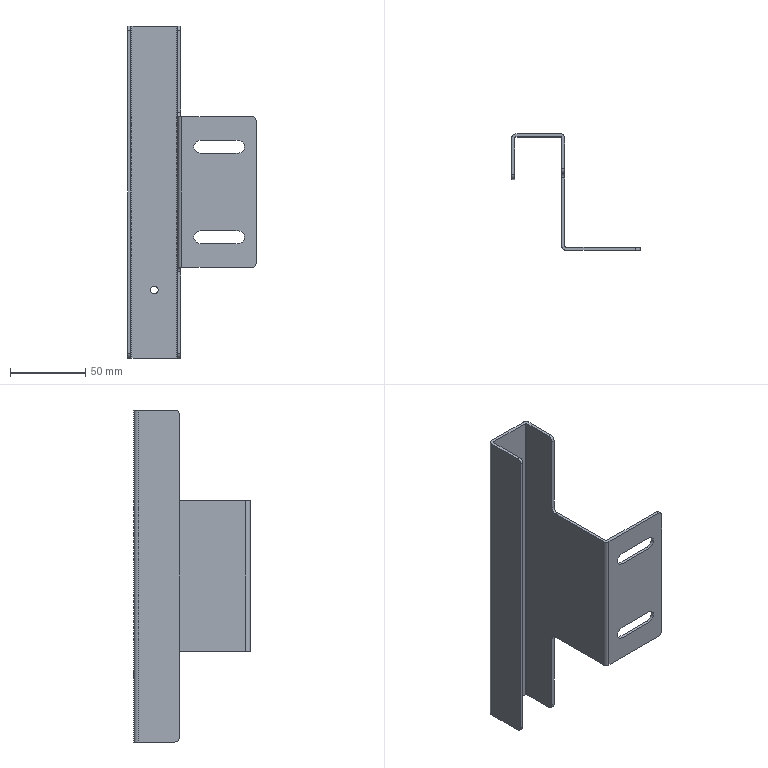Part | SolidWorks | features BaseBody 1 | 1 solid | 40 faces | box 85 x 77 x 220 mm | volume 56604 mm3 | cylinder 20 | plane 20 | commonest cylinder face diameters 6 x8 8.5 x4 1.473 x3 5.473 x3 5 x2
STEP:
#1=CARTESIAN_POINT('',(17.5,-2.,-67.5));
#2=VERTEX_POINT('',#1);
#3=CARTESIAN_POINT('',(17.5,-2.,-62.5));
#4=VERTEX_POINT('',#3);
#5=CARTESIAN_POINT('',(17.5,-2.,-65.));
#6=DIRECTION('',(0.,1.,0.));
#7=DIRECTION('',(0.,0.,1.));
#8=AXIS2_PLACEMENT_3D('',#5,#6,#7);
#9=CIRCLE('',#8,2.5);
#10=EDGE_CURVE('',#2,#4,#9,.T.);
#11=ORIENTED_EDGE('',*,*,#10,.F.);
#12=CARTESIAN_POINT('',(17.5,0.,-67.5));
#13=VERTEX_POINT('',#12);
#14=CARTESIAN_POINT('',(17.5,-10.,-67.5));
#15=DIRECTION('',(0.,1.,0.));
#16=VECTOR('',#15,1000.);
#17=LINE('',#14,#16);
#18=EDGE_CURVE('',#2,#13,#17,.T.);
#19=ORIENTED_EDGE('',*,*,#18,.T.);
#20=CARTESIAN_POINT('',(17.5,0.,-62.5));
#21=VERTEX_POINT('',#20);
#22=CARTESIAN_POINT('',(17.5,0.,-65.));
#23=DIRECTION('',(0.,-1.,0.));
#24=DIRECTION('',(0.,0.,1.));
#25=AXIS2_PLACEMENT_3D('',#22,#23,#24);
#26=CIRCLE('',#25,2.5);
#27=EDGE_CURVE('',#21,#13,#26,.T.);
#28=ORIENTED_EDGE('',*,*,#27,.F.);
#29=CARTESIAN_POINT('',(17.5,-10.,-62.5));
#30=DIRECTION('',(0.,1.,0.));
#31=VECTOR('',#30,1000.);
#32=LINE('',#29,#31);
#33=EDGE_CURVE('',#4,#21,#32,.T.);
#34=ORIENTED_EDGE('',*,*,#33,.F.);
#35=EDGE_LOOP('',(#11,#19,#28,#34));
#36=FACE_OUTER_BOUND('',#35,.T.);
#37=CARTESIAN_POINT('',(17.5,-10.,-65.));
#38=DIRECTION('',(0.,1.,0.));
#39=DIRECTION('',(0.,0.,1.));
#40=AXIS2_PLACEMENT_3D('',#37,#38,#39);
#41=CYLINDRICAL_SURFACE('',#40,2.5);
#42=ADVANCED_FACE('',(#36),#41,.F.);
#43=CARTESIAN_POINT('',(35.,-74.263,-50.));
#44=VERTEX_POINT('',#43);
#45=CARTESIAN_POINT('',(35.,-29.255,-50.));
#46=VERTEX_POINT('',#45);
#47=CARTESIAN_POINT('',(35.,0.,-50.));
#48=DIRECTION('',(0.,1.,0.));
#49=VECTOR('',#48,1000.);
#50=LINE('',#47,#49);
#51=EDGE_CURVE('',#44,#46,#50,.T.);
#52=ORIENTED_EDGE('',*,*,#51,.T.);
#53=CARTESIAN_POINT('',(35.,-26.255,-53.));
#54=VERTEX_POINT('',#53);
#55=CARTESIAN_POINT('',(35.,-29.255,-53.));
#56=DIRECTION('',(-1.,0.,0.));
#57=DIRECTION('',(0.,0.,1.));
#58=AXIS2_PLACEMENT_3D('',#55,#56,#57);
#59=CIRCLE('',#58,3.);
#60=EDGE_CURVE('',#46,#54,#59,.T.);
#61=ORIENTED_EDGE('',*,*,#60,.T.);
#62=CARTESIAN_POINT('',(35.,-26.255,-107.));
#63=VERTEX_POINT('',#62);
#64=CARTESIAN_POINT('',(35.,-26.255,110.));
#65=DIRECTION('',(0.,0.,-1.));
#66=VECTOR('',#65,1000.);
#67=LINE('',#64,#66);
#68=EDGE_CURVE('',#54,#63,#67,.T.);
#69=ORIENTED_EDGE('',*,*,#68,.T.);
#70=CARTESIAN_POINT('',(35.,-23.255,-110.));
#71=VERTEX_POINT('',#70);
#72=CARTESIAN_POINT('',(35.,-23.255,-107.));
#73=DIRECTION('',(1.,0.,0.));
#74=DIRECTION('',(0.,0.,1.));
#75=AXIS2_PLACEMENT_3D('',#72,#73,#74);
#76=CIRCLE('',#75,3.);
#77=EDGE_CURVE('',#63,#71,#76,.T.);
#78=ORIENTED_EDGE('',*,*,#77,.T.);
#79=CARTESIAN_POINT('',(35.,-2.737,-110.));
#80=VERTEX_POINT('',#79);
#81=CARTESIAN_POINT('',(35.,0.,-110.));
#82=DIRECTION('',(0.,1.,0.));
#83=VECTOR('',#82,1000.);
#84=LINE('',#81,#83);
#85=EDGE_CURVE('',#71,#80,#84,.T.);
#86=ORIENTED_EDGE('',*,*,#85,.T.);
#87=CARTESIAN_POINT('',(35.,-2.737,110.));
#88=VERTEX_POINT('',#87);
#89=CARTESIAN_POINT('',(35.,-2.737,110.));
#90=DIRECTION('',(0.,0.,1.));
#91=VECTOR('',#90,1000.);
#92=LINE('',#89,#91);
#93=EDGE_CURVE('',#80,#88,#92,.T.);
#94=ORIENTED_EDGE('',*,*,#93,.T.);
#95=CARTESIAN_POINT('',(35.,-23.255,110.));
#96=VERTEX_POINT('',#95);
#97=CARTESIAN_POINT('',(35.,0.,110.));
#98=DIRECTION('',(0.,-1.,0.));
#99=VECTOR('',#98,1000.);
#100=LINE('',#97,#99);
#101=EDGE_CURVE('',#88,#96,#100,.T.);
#102=ORIENTED_EDGE('',*,*,#101,.T.);
#103=CARTESIAN_POINT('',(35.,-26.255,107.));
#104=VERTEX_POINT('',#103);
#105=CARTESIAN_POINT('',(35.,-23.255,107.));
#106=DIRECTION('',(1.,0.,0.));
#107=DIRECTION('',(0.,0.,1.));
#108=AXIS2_PLACEMENT_3D('',#105,#106,#107);
#109=CIRCLE('',#108,3.);
#110=EDGE_CURVE('',#96,#104,#109,.T.);
#111=ORIENTED_EDGE('',*,*,#110,.T.);
#112=CARTESIAN_POINT('',(35.,-26.255,53.));
#113=VERTEX_POINT('',#112);
#114=CARTESIAN_POINT('',(35.,-26.255,110.));
#115=DIRECTION('',(0.,0.,-1.));
#116=VECTOR('',#115,1000.);
#117=LINE('',#114,#116);
#118=EDGE_CURVE('',#104,#113,#117,.T.);
#119=ORIENTED_EDGE('',*,*,#118,.T.);
#120=CARTESIAN_POINT('',(35.,-29.255,50.));
#121=VERTEX_POINT('',#120);
#122=CARTESIAN_POINT('',(35.,-29.255,53.));
#123=DIRECTION('',(-1.,0.,0.));
#124=DIRECTION('',(0.,0.,1.));
#125=AXIS2_PLACEMENT_3D('',#122,#123,#124);
#126=CIRCLE('',#125,3.);
#127=EDGE_CURVE('',#113,#121,#126,.T.);
#128=ORIENTED_EDGE('',*,*,#127,.T.);
#129=CARTESIAN_POINT('',(35.,-74.263,50.));
#130=VERTEX_POINT('',#129);
#131=CARTESIAN_POINT('',(35.,0.,50.));
#132=DIRECTION('',(0.,-1.,0.));
#133=VECTOR('',#132,1000.);
#134=LINE('',#131,#133);
#135=EDGE_CURVE('',#121,#130,#134,.T.);
#136=ORIENTED_EDGE('',*,*,#135,.T.);
#137=CARTESIAN_POINT('',(35.,-74.263,110.));
#138=DIRECTION('',(0.,0.,-1.));
#139=VECTOR('',#138,1000.);
#140=LINE('',#137,#139);
#141=EDGE_CURVE('',#130,#44,#140,.T.);
#142=ORIENTED_EDGE('',*,*,#141,.T.);
#143=EDGE_LOOP('',(#52,#61,#69,#78,#86,#94,#102,#111,#119,#128,#136,#142));
#144=FACE_OUTER_BOUND('',#143,.T.);
#145=CARTESIAN_POINT('',(35.,0.,110.));
#146=DIRECTION('',(1.,0.,0.));
#147=DIRECTION('',(0.,0.,-1.));
#148=AXIS2_PLACEMENT_3D('',#145,#146,#147);
#149=PLANE('',#148);
#150=ADVANCED_FACE('',(#144),#149,.T.);
#151=CARTESIAN_POINT('',(33.,-26.255,-53.));
#152=VERTEX_POINT('',#151);
#153=CARTESIAN_POINT('',(25.,-26.255,-53.));
#154=DIRECTION('',(-1.,0.,0.));
#155=VECTOR('',#154,1000.);
#156=LINE('',#153,#155);
#157=EDGE_CURVE('',#54,#152,#156,.T.);
#158=ORIENTED_EDGE('',*,*,#157,.F.);
#159=ORIENTED_EDGE('',*,*,#60,.F.);
#160=CARTESIAN_POINT('',(33.,-29.255,-50.));
#161=VERTEX_POINT('',#160);
#162=CARTESIAN_POINT('',(25.,-29.255,-50.));
#163=DIRECTION('',(1.,0.,0.));
#164=VECTOR('',#163,1000.);
#165=LINE('',#162,#164);
#166=EDGE_CURVE('',#161,#46,#165,.T.);
#167=ORIENTED_EDGE('',*,*,#166,.F.);
#168=CARTESIAN_POINT('',(33.,-29.255,-53.));
#169=DIRECTION('',(1.,0.,0.));
#170=DIRECTION('',(0.,0.,1.));
#171=AXIS2_PLACEMENT_3D('',#168,#169,#170);
#172=CIRCLE('',#171,3.);
#173=EDGE_CURVE('',#152,#161,#172,.T.);
#174=ORIENTED_EDGE('',*,*,#173,.F.);
#175=EDGE_LOOP('',(#158,#159,#167,#174));
#176=FACE_OUTER_BOUND('',#175,.T.);
#177=CARTESIAN_POINT('',(25.,-29.255,-53.));
#178=DIRECTION('',(-1.,0.,0.));
#179=DIRECTION('',(0.,0.,1.));
#180=AXIS2_PLACEMENT_3D('',#177,#178,#179);
#181=CYLINDRICAL_SURFACE('',#180,3.);
#182=ADVANCED_FACE('',(#176),#181,.F.);
#183=ORIENTED_EDGE('',*,*,#166,.T.);
#184=ORIENTED_EDGE('',*,*,#51,.F.);
#185=CARTESIAN_POINT('',(35.737,-75.,-50.));
#186=VERTEX_POINT('',#185);
#187=CARTESIAN_POINT('',(35.737,-74.263,-50.));
#188=DIRECTION('',(0.,0.,1.));
#189=DIRECTION('',(-1.,0.,0.));
#190=AXIS2_PLACEMENT_3D('',#187,#188,#189);
#191=CIRCLE('',#190,0.7366);
#192=EDGE_CURVE('',#44,#186,#191,.T.);
#193=ORIENTED_EDGE('',*,*,#192,.T.);
#194=CARTESIAN_POINT('',(82.,-75.,-50.));
#195=VERTEX_POINT('',#194);
#196=CARTESIAN_POINT('',(35.,-75.,-50.));
#197=DIRECTION('',(-1.,0.,0.));
#198=VECTOR('',#197,1000.);
#199=LINE('',#196,#198);
#200=EDGE_CURVE('',#195,#186,#199,.T.);
#201=ORIENTED_EDGE('',*,*,#200,.F.);
#202=CARTESIAN_POINT('',(82.,-77.,-50.));
#203=VERTEX_POINT('',#202);
#204=CARTESIAN_POINT('',(82.,-85.,-50.));
#205=DIRECTION('',(0.,1.,0.));
#206=VECTOR('',#205,1000.);
#207=LINE('',#204,#206);
#208=EDGE_CURVE('',#203,#195,#207,.T.);
#209=ORIENTED_EDGE('',*,*,#208,.F.);
#210=CARTESIAN_POINT('',(35.737,-77.,-50.));
#211=VERTEX_POINT('',#210);
#212=CARTESIAN_POINT('',(85.,-77.,-50.));
#213=DIRECTION('',(1.,0.,0.));
#214=VECTOR('',#213,1000.);
#215=LINE('',#212,#214);
#216=EDGE_CURVE('',#211,#203,#215,.T.);
#217=ORIENTED_EDGE('',*,*,#216,.F.);
#218=CARTESIAN_POINT('',(33.,-74.263,-50.));
#219=VERTEX_POINT('',#218);
#220=CARTESIAN_POINT('',(35.737,-74.263,-50.));
#221=DIRECTION('',(0.,0.,1.));
#222=DIRECTION('',(-1.,0.,0.));
#223=AXIS2_PLACEMENT_3D('',#220,#221,#222);
#224=CIRCLE('',#223,2.737);
#225=EDGE_CURVE('',#219,#211,#224,.T.);
#226=ORIENTED_EDGE('',*,*,#225,.F.);
#227=CARTESIAN_POINT('',(33.,-126.255,-50.));
#228=DIRECTION('',(0.,-1.,0.));
#229=VECTOR('',#228,1000.);
#230=LINE('',#227,#229);
#231=EDGE_CURVE('',#161,#219,#230,.T.);
#232=ORIENTED_EDGE('',*,*,#231,.F.);
#233=EDGE_LOOP('',(#183,#184,#193,#201,#209,#217,#226,#232));
#234=FACE_OUTER_BOUND('',#233,.T.);
#235=CARTESIAN_POINT('',(25.,-126.255,-50.));
#236=DIRECTION('',(0.,0.,1.));
#237=DIRECTION('',(1.,0.,0.));
#238=AXIS2_PLACEMENT_3D('',#235,#236,#237);
#239=PLANE('',#238);
#240=ADVANCED_FACE('',(#234),#239,.F.);
#241=ORIENTED_EDGE('',*,*,#141,.F.);
#242=CARTESIAN_POINT('',(35.737,-75.,50.));
#243=VERTEX_POINT('',#242);
#244=CARTESIAN_POINT('',(35.737,-74.263,50.));
#245=DIRECTION('',(0.,0.,1.));
#246=DIRECTION('',(-1.,0.,0.));
#247=AXIS2_PLACEMENT_3D('',#244,#245,#246);
#248=CIRCLE('',#247,0.7366);
#249=EDGE_CURVE('',#130,#243,#248,.T.);
#250=ORIENTED_EDGE('',*,*,#249,.T.);
#251=CARTESIAN_POINT('',(35.737,-75.,100.057));
#252=DIRECTION('',(0.,0.,1.));
#253=VECTOR('',#252,1000.);
#254=LINE('',#251,#253);
#255=EDGE_CURVE('',#186,#243,#254,.T.);
#256=ORIENTED_EDGE('',*,*,#255,.F.);
#257=ORIENTED_EDGE('',*,*,#192,.F.);
#258=EDGE_LOOP('',(#241,#250,#256,#257));
#259=FACE_OUTER_BOUND('',#258,.T.);
#260=CARTESIAN_POINT('',(35.737,-74.263,100.057));
#261=DIRECTION('',(0.,0.,-1.));
#262=DIRECTION('',(-1.,0.,0.));
#263=AXIS2_PLACEMENT_3D('',#260,#261,#262);
#264=CYLINDRICAL_SURFACE('',#263,0.7366);
#265=ADVANCED_FACE('',(#259),#264,.F.);
#266=CARTESIAN_POINT('',(33.,-29.255,50.));
#267=VERTEX_POINT('',#266);
#268=CARTESIAN_POINT('',(25.,-29.255,50.));
#269=DIRECTION('',(1.,0.,0.));
#270=VECTOR('',#269,1000.);
#271=LINE('',#268,#270);
#272=EDGE_CURVE('',#267,#121,#271,.T.);
#273=ORIENTED_EDGE('',*,*,#272,.F.);
#274=CARTESIAN_POINT('',(33.,-74.263,50.));
#275=VERTEX_POINT('',#274);
#276=CARTESIAN_POINT('',(33.,-126.255,50.));
#277=DIRECTION('',(0.,1.,0.));
#278=VECTOR('',#277,1000.);
#279=LINE('',#276,#278);
#280=EDGE_CURVE('',#275,#267,#279,.T.);
#281=ORIENTED_EDGE('',*,*,#280,.F.);
#282=CARTESIAN_POINT('',(35.737,-77.,50.));
#283=VERTEX_POINT('',#282);
#284=CARTESIAN_POINT('',(35.737,-74.263,50.));
#285=DIRECTION('',(0.,0.,-1.));
#286=DIRECTION('',(-1.,0.,0.));
#287=AXIS2_PLACEMENT_3D('',#284,#285,#286);
#288=CIRCLE('',#287,2.737);
#289=EDGE_CURVE('',#283,#275,#288,.T.);
#290=ORIENTED_EDGE('',*,*,#289,.F.);
#291=CARTESIAN_POINT('',(82.,-77.,50.));
#292=VERTEX_POINT('',#291);
#293=CARTESIAN_POINT('',(85.,-77.,50.));
#294=DIRECTION('',(-1.,0.,0.));
#295=VECTOR('',#294,1000.);
#296=LINE('',#293,#295);
#297=EDGE_CURVE('',#292,#283,#296,.T.);
#298=ORIENTED_EDGE('',*,*,#297,.F.);
#299=CARTESIAN_POINT('',(82.,-75.,50.));
#300=VERTEX_POINT('',#299);
#301=CARTESIAN_POINT('',(82.,-85.,50.));
#302=DIRECTION('',(0.,-1.,0.));
#303=VECTOR('',#302,1000.);
#304=LINE('',#301,#303);
#305=EDGE_CURVE('',#300,#292,#304,.T.);
#306=ORIENTED_EDGE('',*,*,#305,.F.);
#307=CARTESIAN_POINT('',(35.,-75.,50.));
#308=DIRECTION('',(1.,0.,0.));
#309=VECTOR('',#308,1000.);
#310=LINE('',#307,#309);
#311=EDGE_CURVE('',#243,#300,#310,.T.);
#312=ORIENTED_EDGE('',*,*,#311,.F.);
#313=ORIENTED_EDGE('',*,*,#249,.F.);
#314=ORIENTED_EDGE('',*,*,#135,.F.);
#315=EDGE_LOOP('',(#273,#281,#290,#298,#306,#312,#313,#314));
#316=FACE_OUTER_BOUND('',#315,.T.);
#317=CARTESIAN_POINT('',(25.,-126.255,50.));
#318=DIRECTION('',(0.,0.,-1.));
#319=DIRECTION('',(0.,1.,0.));
#320=AXIS2_PLACEMENT_3D('',#317,#318,#319);
#321=PLANE('',#320);
#322=ADVANCED_FACE('',(#316),#321,.F.);
#323=ORIENTED_EDGE('',*,*,#272,.T.);
#324=ORIENTED_EDGE('',*,*,#127,.F.);
#325=CARTESIAN_POINT('',(33.,-26.255,53.));
#326=VERTEX_POINT('',#325);
#327=CARTESIAN_POINT('',(25.,-26.255,53.));
#328=DIRECTION('',(1.,0.,0.));
#329=VECTOR('',#328,1000.);
#330=LINE('',#327,#329);
#331=EDGE_CURVE('',#326,#113,#330,.T.);
#332=ORIENTED_EDGE('',*,*,#331,.F.);
#333=CARTESIAN_POINT('',(33.,-29.255,53.));
#334=DIRECTION('',(1.,0.,0.));
#335=DIRECTION('',(0.,0.,1.));
#336=AXIS2_PLACEMENT_3D('',#333,#334,#335);
#337=CIRCLE('',#336,3.);
#338=EDGE_CURVE('',#267,#326,#337,.T.);
#339=ORIENTED_EDGE('',*,*,#338,.F.);
#340=EDGE_LOOP('',(#323,#324,#332,#339));
#341=FACE_OUTER_BOUND('',#340,.T.);
#342=CARTESIAN_POINT('',(25.,-29.255,53.));
#343=DIRECTION('',(-1.,0.,0.));
#344=DIRECTION('',(0.,0.,1.));
#345=AXIS2_PLACEMENT_3D('',#342,#343,#344);
#346=CYLINDRICAL_SURFACE('',#345,3.);
#347=ADVANCED_FACE('',(#341),#346,.F.);
#348=ORIENTED_EDGE('',*,*,#331,.T.);
#349=ORIENTED_EDGE('',*,*,#118,.F.);
#350=CARTESIAN_POINT('',(33.,-26.255,107.));
#351=VERTEX_POINT('',#350);
#352=CARTESIAN_POINT('',(25.,-26.255,107.));
#353=DIRECTION('',(1.,0.,0.));
#354=VECTOR('',#353,1000.);
#355=LINE('',#352,#354);
#356=EDGE_CURVE('',#351,#104,#355,.T.);
#357=ORIENTED_EDGE('',*,*,#356,.F.);
#358=CARTESIAN_POINT('',(33.,-26.255,110.));
#359=DIRECTION('',(0.,0.,1.));
#360=VECTOR('',#359,1000.);
#361=LINE('',#358,#360);
#362=EDGE_CURVE('',#326,#351,#361,.T.);
#363=ORIENTED_EDGE('',*,*,#362,.F.);
#364=EDGE_LOOP('',(#348,#349,#357,#363));
#365=FACE_OUTER_BOUND('',#364,.T.);
#366=CARTESIAN_POINT('',(25.,-26.255,110.));
#367=DIRECTION('',(0.,1.,0.));
#368=DIRECTION('',(0.,0.,1.));
#369=AXIS2_PLACEMENT_3D('',#366,#367,#368);
#370=PLANE('',#369);
#371=ADVANCED_FACE('',(#365),#370,.F.);
#372=ORIENTED_EDGE('',*,*,#110,.F.);
#373=CARTESIAN_POINT('',(33.,-23.255,110.));
#374=VERTEX_POINT('',#373);
#375=CARTESIAN_POINT('',(32.263,-23.255,110.));
#376=DIRECTION('',(-1.,0.,0.));
#377=VECTOR('',#376,1000.);
#378=LINE('',#375,#377);
#379=EDGE_CURVE('',#96,#374,#378,.T.);
#380=ORIENTED_EDGE('',*,*,#379,.T.);
#381=CARTESIAN_POINT('',(33.,-23.255,107.));
#382=DIRECTION('',(1.,0.,0.));
#383=DIRECTION('',(0.,0.,1.));
#384=AXIS2_PLACEMENT_3D('',#381,#382,#383);
#385=CIRCLE('',#384,3.);
#386=EDGE_CURVE('',#374,#351,#385,.T.);
#387=ORIENTED_EDGE('',*,*,#386,.T.);
#388=ORIENTED_EDGE('',*,*,#356,.T.);
#389=EDGE_LOOP('',(#372,#380,#387,#388));
#390=FACE_OUTER_BOUND('',#389,.T.);
#391=CARTESIAN_POINT('',(32.263,-23.255,107.));
#392=DIRECTION('',(-1.,0.,0.));
#393=DIRECTION('',(0.,0.,1.));
#394=AXIS2_PLACEMENT_3D('',#391,#392,#393);
#395=CYLINDRICAL_SURFACE('',#394,3.);
#396=ADVANCED_FACE('',(#390),#395,.T.);
#397=ORIENTED_EDGE('',*,*,#101,.F.);
#398=CARTESIAN_POINT('',(32.263,0.,110.));
#399=VERTEX_POINT('',#398);
#400=CARTESIAN_POINT('',(32.263,-2.737,110.));
#401=DIRECTION('',(0.,0.,-1.));
#402=DIRECTION('',(-1.,0.,0.));
#403=AXIS2_PLACEMENT_3D('',#400,#401,#402);
#404=CIRCLE('',#403,2.737);
#405=EDGE_CURVE('',#399,#88,#404,.T.);
#406=ORIENTED_EDGE('',*,*,#405,.F.);
#407=CARTESIAN_POINT('',(2.737,0.,110.));
#408=VERTEX_POINT('',#407);
#409=CARTESIAN_POINT('',(0.,0.,110.));
#410=DIRECTION('',(1.,0.,0.));
#411=VECTOR('',#410,1000.);
#412=LINE('',#409,#411);
#413=EDGE_CURVE('',#408,#399,#412,.T.);
#414=ORIENTED_EDGE('',*,*,#413,.F.);
#415=CARTESIAN_POINT('',(0.,-2.737,110.));
#416=VERTEX_POINT('',#415);
#417=CARTESIAN_POINT('',(2.737,-2.737,110.));
#418=DIRECTION('',(0.,0.,-1.));
#419=DIRECTION('',(-1.,0.,0.));
#420=AXIS2_PLACEMENT_3D('',#417,#418,#419);
#421=CIRCLE('',#420,2.737);
#422=EDGE_CURVE('',#416,#408,#421,.T.);
#423=ORIENTED_EDGE('',*,*,#422,.F.);
#424=CARTESIAN_POINT('',(0.,-27.,110.));
#425=VERTEX_POINT('',#424);
#426=CARTESIAN_POINT('',(0.,-30.,110.));
#427=DIRECTION('',(0.,1.,0.));
#428=VECTOR('',#427,1000.);
#429=LINE('',#426,#428);
#430=EDGE_CURVE('',#425,#416,#429,.T.);
#431=ORIENTED_EDGE('',*,*,#430,.F.);
#432=CARTESIAN_POINT('',(2.,-27.,110.));
#433=VERTEX_POINT('',#432);
#434=CARTESIAN_POINT('',(35.737,-27.,110.));
#435=DIRECTION('',(-1.,0.,0.));
#436=VECTOR('',#435,1000.);
#437=LINE('',#434,#436);
#438=EDGE_CURVE('',#433,#425,#437,.T.);
#439=ORIENTED_EDGE('',*,*,#438,.F.);
#440=CARTESIAN_POINT('',(2.,-2.737,110.));
#441=VERTEX_POINT('',#440);
#442=CARTESIAN_POINT('',(2.,-74.263,110.));
#443=DIRECTION('',(0.,-1.,0.));
#444=VECTOR('',#443,1000.);
#445=LINE('',#442,#444);
#446=EDGE_CURVE('',#441,#433,#445,.T.);
#447=ORIENTED_EDGE('',*,*,#446,.F.);
#448=CARTESIAN_POINT('',(2.737,-2.,110.));
#449=VERTEX_POINT('',#448);
#450=CARTESIAN_POINT('',(2.737,-2.737,110.));
#451=DIRECTION('',(0.,0.,-1.));
#452=DIRECTION('',(-1.,0.,0.));
#453=AXIS2_PLACEMENT_3D('',#450,#451,#452);
#454=CIRCLE('',#453,0.7366);
#455=EDGE_CURVE('',#441,#449,#454,.T.);
#456=ORIENTED_EDGE('',*,*,#455,.T.);
#457=CARTESIAN_POINT('',(32.263,-2.,110.));
#458=VERTEX_POINT('',#457);
#459=CARTESIAN_POINT('',(2.,-2.,110.));
#460=DIRECTION('',(1.,0.,0.));
#461=VECTOR('',#460,1000.);
#462=LINE('',#459,#461);
#463=EDGE_CURVE('',#449,#458,#462,.T.);
#464=ORIENTED_EDGE('',*,*,#463,.T.);
#465=CARTESIAN_POINT('',(33.,-2.737,110.));
#466=VERTEX_POINT('',#465);
#467=CARTESIAN_POINT('',(32.263,-2.737,110.));
#468=DIRECTION('',(0.,0.,-1.));
#469=DIRECTION('',(-1.,0.,0.));
#470=AXIS2_PLACEMENT_3D('',#467,#468,#469);
#471=CIRCLE('',#470,0.7366);
#472=EDGE_CURVE('',#458,#466,#471,.T.);
#473=ORIENTED_EDGE('',*,*,#472,.T.);
#474=CARTESIAN_POINT('',(33.,-2.,110.));
#475=DIRECTION('',(0.,-1.,0.));
#476=VECTOR('',#475,1000.);
#477=LINE('',#474,#476);
#478=EDGE_CURVE('',#466,#374,#477,.T.);
#479=ORIENTED_EDGE('',*,*,#478,.T.);
#480=ORIENTED_EDGE('',*,*,#379,.F.);
#481=EDGE_LOOP('',(#397,#406,#414,#423,#431,#439,#447,#456,#464,#473,#479,#480));
#482=FACE_OUTER_BOUND('',#481,.T.);
#483=CARTESIAN_POINT('',(32.263,-2.,110.));
#484=DIRECTION('',(0.,0.,1.));
#485=DIRECTION('',(1.,0.,0.));
#486=AXIS2_PLACEMENT_3D('',#483,#484,#485);
#487=PLANE('',#486);
#488=ADVANCED_FACE('',(#482),#487,.T.);
#489=ORIENTED_EDGE('',*,*,#405,.T.);
#490=ORIENTED_EDGE('',*,*,#93,.F.);
#491=CARTESIAN_POINT('',(32.263,0.,-110.));
#492=VERTEX_POINT('',#491);
#493=CARTESIAN_POINT('',(32.263,-2.737,-110.));
#494=DIRECTION('',(0.,0.,1.));
#495=DIRECTION('',(-1.,0.,0.));
#496=AXIS2_PLACEMENT_3D('',#493,#494,#495);
#497=CIRCLE('',#496,2.737);
#498=EDGE_CURVE('',#80,#492,#497,.T.);
#499=ORIENTED_EDGE('',*,*,#498,.T.);
#500=CARTESIAN_POINT('',(32.263,0.,110.));
#501=DIRECTION('',(0.,0.,1.));
#502=VECTOR('',#501,1000.);
#503=LINE('',#500,#502);
#504=EDGE_CURVE('',#492,#399,#503,.T.);
#505=ORIENTED_EDGE('',*,*,#504,.T.);
#506=EDGE_LOOP('',(#489,#490,#499,#505));
#507=FACE_OUTER_BOUND('',#506,.T.);
#508=CARTESIAN_POINT('',(32.263,-2.737,110.));
#509=DIRECTION('',(0.,0.,-1.));
#510=DIRECTION('',(-1.,0.,0.));
#511=AXIS2_PLACEMENT_3D('',#508,#509,#510);
#512=CYLINDRICAL_SURFACE('',#511,2.737);
#513=ADVANCED_FACE('',(#507),#512,.T.);
#514=CARTESIAN_POINT('',(33.,-23.255,-110.));
#515=VERTEX_POINT('',#514);
#516=CARTESIAN_POINT('',(33.,-2.737,-110.));
#517=VERTEX_POINT('',#516);
#518=CARTESIAN_POINT('',(33.,-77.,-110.));
#519=DIRECTION('',(0.,1.,0.));
#520=VECTOR('',#519,1000.);
#521=LINE('',#518,#520);
#522=EDGE_CURVE('',#515,#517,#521,.T.);
#523=ORIENTED_EDGE('',*,*,#522,.T.);
#524=CARTESIAN_POINT('',(32.263,-2.,-110.));
#525=VERTEX_POINT('',#524);
#526=CARTESIAN_POINT('',(32.263,-2.737,-110.));
#527=DIRECTION('',(0.,0.,1.));
#528=DIRECTION('',(-1.,0.,0.));
#529=AXIS2_PLACEMENT_3D('',#526,#527,#528);
#530=CIRCLE('',#529,0.7366);
#531=EDGE_CURVE('',#517,#525,#530,.T.);
#532=ORIENTED_EDGE('',*,*,#531,.T.);
#533=CARTESIAN_POINT('',(2.737,-2.,-110.));
#534=VERTEX_POINT('',#533);
#535=CARTESIAN_POINT('',(33.,-2.,-110.));
#536=DIRECTION('',(-1.,0.,0.));
#537=VECTOR('',#536,1000.);
#538=LINE('',#535,#537);
#539=EDGE_CURVE('',#525,#534,#538,.T.);
#540=ORIENTED_EDGE('',*,*,#539,.T.);
#541=CARTESIAN_POINT('',(2.,-2.737,-110.));
#542=VERTEX_POINT('',#541);
#543=CARTESIAN_POINT('',(2.737,-2.737,-110.));
#544=DIRECTION('',(0.,0.,1.));
#545=DIRECTION('',(-1.,0.,0.));
#546=AXIS2_PLACEMENT_3D('',#543,#544,#545);
#547=CIRCLE('',#546,0.7366);
#548=EDGE_CURVE('',#534,#542,#547,.T.);
#549=ORIENTED_EDGE('',*,*,#548,.T.);
#550=CARTESIAN_POINT('',(2.,-27.,-110.));
#551=VERTEX_POINT('',#550);
#552=CARTESIAN_POINT('',(2.,-2.,-110.));
#553=DIRECTION('',(0.,-1.,0.));
#554=VECTOR('',#553,1000.);
#555=LINE('',#552,#554);
#556=EDGE_CURVE('',#542,#551,#555,.T.);
#557=ORIENTED_EDGE('',*,*,#556,.T.);
#558=CARTESIAN_POINT('',(0.,-27.,-110.));
#559=VERTEX_POINT('',#558);
#560=CARTESIAN_POINT('',(2.737,-27.,-110.));
#561=DIRECTION('',(1.,0.,0.));
#562=VECTOR('',#561,1000.);
#563=LINE('',#560,#562);
#564=EDGE_CURVE('',#559,#551,#563,.T.);
#565=ORIENTED_EDGE('',*,*,#564,.F.);
#566=CARTESIAN_POINT('',(0.,-2.737,-110.));
#567=VERTEX_POINT('',#566);
#568=CARTESIAN_POINT('',(0.,-30.,-110.));
#569=DIRECTION('',(0.,-1.,0.));
#570=VECTOR('',#569,1000.);
#571=LINE('',#568,#570);
#572=EDGE_CURVE('',#567,#559,#571,.T.);
#573=ORIENTED_EDGE('',*,*,#572,.F.);
#574=CARTESIAN_POINT('',(2.737,0.,-110.));
#575=VERTEX_POINT('',#574);
#576=CARTESIAN_POINT('',(2.737,-2.737,-110.));
#577=DIRECTION('',(0.,0.,1.));
#578=DIRECTION('',(-1.,0.,0.));
#579=AXIS2_PLACEMENT_3D('',#576,#577,#578);
#580=CIRCLE('',#579,2.737);
#581=EDGE_CURVE('',#575,#567,#580,.T.);
#582=ORIENTED_EDGE('',*,*,#581,.F.);
#583=CARTESIAN_POINT('',(0.,0.,-110.));
#584=DIRECTION('',(-1.,0.,0.));
#585=VECTOR('',#584,1000.);
#586=LINE('',#583,#585);
#587=EDGE_CURVE('',#492,#575,#586,.T.);
#588=ORIENTED_EDGE('',*,*,#587,.F.);
#589=ORIENTED_EDGE('',*,*,#498,.F.);
#590=ORIENTED_EDGE('',*,*,#85,.F.);
#591=CARTESIAN_POINT('',(35.737,-23.255,-110.));
#592=DIRECTION('',(-1.,0.,0.));
#593=VECTOR('',#592,1000.);
#594=LINE('',#591,#593);
#595=EDGE_CURVE('',#71,#515,#594,.T.);
#596=ORIENTED_EDGE('',*,*,#595,.T.);
#597=EDGE_LOOP('',(#523,#532,#540,#549,#557,#565,#573,#582,#588,#589,#590,#596));
#598=FACE_OUTER_BOUND('',#597,.T.);
#599=CARTESIAN_POINT('',(35.737,-77.,-110.));
#600=DIRECTION('',(0.,0.,-1.));
#601=DIRECTION('',(-1.,0.,0.));
#602=AXIS2_PLACEMENT_3D('',#599,#600,#601);
#603=PLANE('',#602);
#604=ADVANCED_FACE('',(#598),#603,.T.);
#605=ORIENTED_EDGE('',*,*,#77,.F.);
#606=CARTESIAN_POINT('',(33.,-26.255,-107.));
#607=VERTEX_POINT('',#606);
#608=CARTESIAN_POINT('',(25.,-26.255,-107.));
#609=DIRECTION('',(-1.,0.,0.));
#610=VECTOR('',#609,1000.);
#611=LINE('',#608,#610);
#612=EDGE_CURVE('',#63,#607,#611,.T.);
#613=ORIENTED_EDGE('',*,*,#612,.T.);
#614=CARTESIAN_POINT('',(33.,-23.255,-107.));
#615=DIRECTION('',(1.,0.,0.));
#616=DIRECTION('',(0.,0.,1.));
#617=AXIS2_PLACEMENT_3D('',#614,#615,#616);
#618=CIRCLE('',#617,3.);
#619=EDGE_CURVE('',#607,#515,#618,.T.);
#620=ORIENTED_EDGE('',*,*,#619,.T.);
#621=ORIENTED_EDGE('',*,*,#595,.F.);
#622=EDGE_LOOP('',(#605,#613,#620,#621));
#623=FACE_OUTER_BOUND('',#622,.T.);
#624=CARTESIAN_POINT('',(25.,-23.255,-107.));
#625=DIRECTION('',(-1.,0.,0.));
#626=DIRECTION('',(0.,0.,1.));
#627=AXIS2_PLACEMENT_3D('',#624,#625,#626);
#628=CYLINDRICAL_SURFACE('',#627,3.);
#629=ADVANCED_FACE('',(#623),#628,.T.);
#630=ORIENTED_EDGE('',*,*,#612,.F.);
#631=ORIENTED_EDGE('',*,*,#68,.F.);
#632=ORIENTED_EDGE('',*,*,#157,.T.);
#633=CARTESIAN_POINT('',(33.,-26.255,-110.));
#634=DIRECTION('',(0.,0.,1.));
#635=VECTOR('',#634,1000.);
#636=LINE('',#633,#635);
#637=EDGE_CURVE('',#607,#152,#636,.T.);
#638=ORIENTED_EDGE('',*,*,#637,.F.);
#639=EDGE_LOOP('',(#630,#631,#632,#638));
#640=FACE_OUTER_BOUND('',#639,.T.);
#641=CARTESIAN_POINT('',(25.,-26.255,-110.));
#642=DIRECTION('',(0.,1.,0.));
#643=DIRECTION('',(0.,0.,1.));
#644=AXIS2_PLACEMENT_3D('',#641,#642,#643);
#645=PLANE('',#644);
#646=ADVANCED_FACE('',(#640),#645,.F.);
#647=ORIENTED_EDGE('',*,*,#619,.F.);
#648=ORIENTED_EDGE('',*,*,#637,.T.);
#649=ORIENTED_EDGE('',*,*,#173,.T.);
#650=ORIENTED_EDGE('',*,*,#231,.T.);
#651=CARTESIAN_POINT('',(33.,-74.263,110.));
#652=DIRECTION('',(0.,0.,-1.));
#653=VECTOR('',#652,1000.);
#654=LINE('',#651,#653);
#655=EDGE_CURVE('',#275,#219,#654,.T.);
#656=ORIENTED_EDGE('',*,*,#655,.F.);
#657=ORIENTED_EDGE('',*,*,#280,.T.);
#658=ORIENTED_EDGE('',*,*,#338,.T.);
#659=ORIENTED_EDGE('',*,*,#362,.T.);
#660=ORIENTED_EDGE('',*,*,#386,.F.);
#661=ORIENTED_EDGE('',*,*,#478,.F.);
#662=CARTESIAN_POINT('',(33.,-2.737,110.));
#663=DIRECTION('',(0.,0.,1.));
#664=VECTOR('',#663,1000.);
#665=LINE('',#662,#664);
#666=EDGE_CURVE('',#517,#466,#665,.T.);
#667=ORIENTED_EDGE('',*,*,#666,.F.);
#668=ORIENTED_EDGE('',*,*,#522,.F.);
#669=EDGE_LOOP('',(#647,#648,#649,#650,#656,#657,#658,#659,#660,#661,#667,#668));
#670=FACE_OUTER_BOUND('',#669,.T.);
#671=CARTESIAN_POINT('',(33.,0.,110.));
#672=DIRECTION('',(1.,0.,0.));
#673=DIRECTION('',(0.,0.,-1.));
#674=AXIS2_PLACEMENT_3D('',#671,#672,#673);
#675=PLANE('',#674);
#676=ADVANCED_FACE('',(#670),#675,.F.);
#677=ORIENTED_EDGE('',*,*,#311,.T.);
#678=CARTESIAN_POINT('',(85.,-75.,47.));
#679=VERTEX_POINT('',#678);
#680=CARTESIAN_POINT('',(82.,-75.,47.));
#681=DIRECTION('',(0.,1.,0.));
#682=DIRECTION('',(0.,0.,-1.));
#683=AXIS2_PLACEMENT_3D('',#680,#681,#682);
#684=CIRCLE('',#683,3.);
#685=EDGE_CURVE('',#300,#679,#684,.T.);
#686=ORIENTED_EDGE('',*,*,#685,.T.);
#687=CARTESIAN_POINT('',(85.,-75.,-47.));
#688=VERTEX_POINT('',#687);
#689=CARTESIAN_POINT('',(85.,-75.,110.));
#690=DIRECTION('',(0.,0.,-1.));
#691=VECTOR('',#690,1000.);
#692=LINE('',#689,#691);
#693=EDGE_CURVE('',#679,#688,#692,.T.);
#694=ORIENTED_EDGE('',*,*,#693,.T.);
#695=CARTESIAN_POINT('',(82.,-75.,-47.));
#696=DIRECTION('',(0.,1.,0.));
#697=DIRECTION('',(0.,0.,-1.));
#698=AXIS2_PLACEMENT_3D('',#695,#696,#697);
#699=CIRCLE('',#698,3.);
#700=EDGE_CURVE('',#688,#195,#699,.T.);
#701=ORIENTED_EDGE('',*,*,#700,.T.);
#702=ORIENTED_EDGE('',*,*,#200,.T.);
#703=ORIENTED_EDGE('',*,*,#255,.T.);
#704=EDGE_LOOP('',(#677,#686,#694,#701,#702,#703));
#705=FACE_OUTER_BOUND('',#704,.T.);
#706=CARTESIAN_POINT('',(73.,-75.,25.75));
#707=VERTEX_POINT('',#706);
#708=CARTESIAN_POINT('',(73.,-75.,34.25));
#709=VERTEX_POINT('',#708);
#710=CARTESIAN_POINT('',(73.,-75.,30.));
#711=DIRECTION('',(0.,-1.,0.));
#712=DIRECTION('',(0.,0.,1.));
#713=AXIS2_PLACEMENT_3D('',#710,#711,#712);
#714=CIRCLE('',#713,4.25);
#715=EDGE_CURVE('',#707,#709,#714,.T.);
#716=ORIENTED_EDGE('',*,*,#715,.T.);
#717=CARTESIAN_POINT('',(48.,-75.,34.25));
#718=VERTEX_POINT('',#717);
#719=CARTESIAN_POINT('',(35.,-75.,34.25));
#720=DIRECTION('',(-1.,0.,0.));
#721=VECTOR('',#720,1000.);
#722=LINE('',#719,#721);
#723=EDGE_CURVE('',#709,#718,#722,.T.);
#724=ORIENTED_EDGE('',*,*,#723,.T.);
#725=CARTESIAN_POINT('',(48.,-75.,25.75));
#726=VERTEX_POINT('',#725);
#727=CARTESIAN_POINT('',(48.,-75.,30.));
#728=DIRECTION('',(0.,-1.,0.));
#729=DIRECTION('',(0.,0.,1.));
#730=AXIS2_PLACEMENT_3D('',#727,#728,#729);
#731=CIRCLE('',#730,4.25);
#732=EDGE_CURVE('',#718,#726,#731,.T.);
#733=ORIENTED_EDGE('',*,*,#732,.T.);
#734=CARTESIAN_POINT('',(35.,-75.,25.75));
#735=DIRECTION('',(1.,0.,0.));
#736=VECTOR('',#735,1000.);
#737=LINE('',#734,#736);
#738=EDGE_CURVE('',#726,#707,#737,.T.);
#739=ORIENTED_EDGE('',*,*,#738,.T.);
#740=EDGE_LOOP('',(#716,#724,#733,#739));
#741=FACE_BOUND('',#740,.T.);
#742=CARTESIAN_POINT('',(73.,-75.,-34.25));
#743=VERTEX_POINT('',#742);
#744=CARTESIAN_POINT('',(73.,-75.,-25.75));
#745=VERTEX_POINT('',#744);
#746=CARTESIAN_POINT('',(73.,-75.,-30.));
#747=DIRECTION('',(0.,-1.,0.));
#748=DIRECTION('',(0.,0.,1.));
#749=AXIS2_PLACEMENT_3D('',#746,#747,#748);
#750=CIRCLE('',#749,4.25);
#751=EDGE_CURVE('',#743,#745,#750,.T.);
#752=ORIENTED_EDGE('',*,*,#751,.T.);
#753=CARTESIAN_POINT('',(48.,-75.,-25.75));
#754=VERTEX_POINT('',#753);
#755=CARTESIAN_POINT('',(35.,-75.,-25.75));
#756=DIRECTION('',(-1.,0.,0.));
#757=VECTOR('',#756,1000.);
#758=LINE('',#755,#757);
#759=EDGE_CURVE('',#745,#754,#758,.T.);
#760=ORIENTED_EDGE('',*,*,#759,.T.);
#761=CARTESIAN_POINT('',(48.,-75.,-34.25));
#762=VERTEX_POINT('',#761);
#763=CARTESIAN_POINT('',(48.,-75.,-30.));
#764=DIRECTION('',(0.,-1.,0.));
#765=DIRECTION('',(0.,0.,1.));
#766=AXIS2_PLACEMENT_3D('',#763,#764,#765);
#767=CIRCLE('',#766,4.25);
#768=EDGE_CURVE('',#754,#762,#767,.T.);
#769=ORIENTED_EDGE('',*,*,#768,.T.);
#770=CARTESIAN_POINT('',(35.,-75.,-34.25));
#771=DIRECTION('',(1.,0.,0.));
#772=VECTOR('',#771,1000.);
#773=LINE('',#770,#772);
#774=EDGE_CURVE('',#762,#743,#773,.T.);
#775=ORIENTED_EDGE('',*,*,#774,.T.);
#776=EDGE_LOOP('',(#752,#760,#769,#775));
#777=FACE_BOUND('',#776,.T.);
#778=CARTESIAN_POINT('',(35.,-75.,110.));
#779=DIRECTION('',(0.,1.,0.));
#780=DIRECTION('',(0.,0.,1.));
#781=AXIS2_PLACEMENT_3D('',#778,#779,#780);
#782=PLANE('',#781);
#783=ADVANCED_FACE('',(#705,#741,#777),#782,.T.);
#784=ORIENTED_EDGE('',*,*,#413,.T.);
#785=ORIENTED_EDGE('',*,*,#504,.F.);
#786=ORIENTED_EDGE('',*,*,#587,.T.);
#787=CARTESIAN_POINT('',(2.737,0.,110.));
#788=DIRECTION('',(0.,0.,1.));
#789=VECTOR('',#788,1000.);
#790=LINE('',#787,#789);
#791=EDGE_CURVE('',#575,#408,#790,.T.);
#792=ORIENTED_EDGE('',*,*,#791,.T.);
#793=EDGE_LOOP('',(#784,#785,#786,#792));
#794=FACE_OUTER_BOUND('',#793,.T.);
#795=ORIENTED_EDGE('',*,*,#27,.T.);
#796=CARTESIAN_POINT('',(17.5,0.,-65.));
#797=DIRECTION('',(0.,-1.,0.));
#798=DIRECTION('',(0.,0.,1.));
#799=AXIS2_PLACEMENT_3D('',#796,#797,#798);
#800=CIRCLE('',#799,2.5);
#801=EDGE_CURVE('',#13,#21,#800,.T.);
#802=ORIENTED_EDGE('',*,*,#801,.T.);
#803=EDGE_LOOP('',(#795,#802));
#804=FACE_BOUND('',#803,.T.);
#805=CARTESIAN_POINT('',(0.,0.,110.));
#806=DIRECTION('',(0.,1.,0.));
#807=DIRECTION('',(0.,0.,1.));
#808=AXIS2_PLACEMENT_3D('',#805,#806,#807);
#809=PLANE('',#808);
#810=ADVANCED_FACE('',(#794,#804),#809,.T.);
#811=ORIENTED_EDGE('',*,*,#289,.T.);
#812=ORIENTED_EDGE('',*,*,#655,.T.);
#813=ORIENTED_EDGE('',*,*,#225,.T.);
#814=CARTESIAN_POINT('',(35.737,-77.,100.057));
#815=DIRECTION('',(0.,0.,1.));
#816=VECTOR('',#815,1000.);
#817=LINE('',#814,#816);
#818=EDGE_CURVE('',#211,#283,#817,.T.);
#819=ORIENTED_EDGE('',*,*,#818,.T.);
#820=EDGE_LOOP('',(#811,#812,#813,#819));
#821=FACE_OUTER_BOUND('',#820,.T.);
#822=CARTESIAN_POINT('',(35.737,-74.263,100.057));
#823=DIRECTION('',(0.,0.,-1.));
#824=DIRECTION('',(-1.,0.,0.));
#825=AXIS2_PLACEMENT_3D('',#822,#823,#824);
#826=CYLINDRICAL_SURFACE('',#825,2.737);
#827=ADVANCED_FACE('',(#821),#826,.T.);
#828=ORIENTED_EDGE('',*,*,#666,.T.);
#829=ORIENTED_EDGE('',*,*,#472,.F.);
#830=CARTESIAN_POINT('',(32.263,-2.,110.));
#831=DIRECTION('',(0.,0.,1.));
#832=VECTOR('',#831,1000.);
#833=LINE('',#830,#832);
#834=EDGE_CURVE('',#525,#458,#833,.T.);
#835=ORIENTED_EDGE('',*,*,#834,.F.);
#836=ORIENTED_EDGE('',*,*,#531,.F.);
#837=EDGE_LOOP('',(#828,#829,#835,#836));
#838=FACE_OUTER_BOUND('',#837,.T.);
#839=CARTESIAN_POINT('',(32.263,-2.737,110.));
#840=DIRECTION('',(0.,0.,-1.));
#841=DIRECTION('',(-1.,0.,0.));
#842=AXIS2_PLACEMENT_3D('',#839,#840,#841);
#843=CYLINDRICAL_SURFACE('',#842,0.7366);
#844=ADVANCED_FACE('',(#838),#843,.F.);
#845=ORIENTED_EDGE('',*,*,#685,.F.);
#846=ORIENTED_EDGE('',*,*,#305,.T.);
#847=CARTESIAN_POINT('',(85.,-77.,47.));
#848=VERTEX_POINT('',#847);
#849=CARTESIAN_POINT('',(82.,-77.,47.));
#850=DIRECTION('',(0.,1.,0.));
#851=DIRECTION('',(0.,0.,-1.));
#852=AXIS2_PLACEMENT_3D('',#849,#850,#851);
#853=CIRCLE('',#852,3.);
#854=EDGE_CURVE('',#292,#848,#853,.T.);
#855=ORIENTED_EDGE('',*,*,#854,.T.);
#856=CARTESIAN_POINT('',(85.,-85.,47.));
#857=DIRECTION('',(0.,1.,0.));
#858=VECTOR('',#857,1000.);
#859=LINE('',#856,#858);
#860=EDGE_CURVE('',#848,#679,#859,.T.);
#861=ORIENTED_EDGE('',*,*,#860,.T.);
#862=EDGE_LOOP('',(#845,#846,#855,#861));
#863=FACE_OUTER_BOUND('',#862,.T.);
#864=CARTESIAN_POINT('',(82.,-85.,47.));
#865=DIRECTION('',(0.,-1.,0.));
#866=DIRECTION('',(0.,0.,-1.));
#867=AXIS2_PLACEMENT_3D('',#864,#865,#866);
#868=CYLINDRICAL_SURFACE('',#867,3.);
#869=ADVANCED_FACE('',(#863),#868,.T.);
#870=ORIENTED_EDGE('',*,*,#700,.F.);
#871=CARTESIAN_POINT('',(85.,-77.,-47.));
#872=VERTEX_POINT('',#871);
#873=CARTESIAN_POINT('',(85.,-75.,-47.));
#874=DIRECTION('',(0.,-1.,0.));
#875=VECTOR('',#874,1000.);
#876=LINE('',#873,#875);
#877=EDGE_CURVE('',#688,#872,#876,.T.);
#878=ORIENTED_EDGE('',*,*,#877,.T.);
#879=CARTESIAN_POINT('',(82.,-77.,-47.));
#880=DIRECTION('',(0.,1.,0.));
#881=DIRECTION('',(0.,0.,-1.));
#882=AXIS2_PLACEMENT_3D('',#879,#880,#881);
#883=CIRCLE('',#882,3.);
#884=EDGE_CURVE('',#872,#203,#883,.T.);
#885=ORIENTED_EDGE('',*,*,#884,.T.);
#886=ORIENTED_EDGE('',*,*,#208,.T.);
#887=EDGE_LOOP('',(#870,#878,#885,#886));
#888=FACE_OUTER_BOUND('',#887,.T.);
#889=CARTESIAN_POINT('',(82.,-75.,-47.));
#890=DIRECTION('',(0.,-1.,0.));
#891=DIRECTION('',(0.,0.,-1.));
#892=AXIS2_PLACEMENT_3D('',#889,#890,#891);
#893=CYLINDRICAL_SURFACE('',#892,3.);
#894=ADVANCED_FACE('',(#888),#893,.T.);
#895=ORIENTED_EDGE('',*,*,#693,.F.);
#896=ORIENTED_EDGE('',*,*,#860,.F.);
#897=CARTESIAN_POINT('',(85.,-77.,110.));
#898=DIRECTION('',(0.,0.,-1.));
#899=VECTOR('',#898,1000.);
#900=LINE('',#897,#899);
#901=EDGE_CURVE('',#848,#872,#900,.T.);
#902=ORIENTED_EDGE('',*,*,#901,.T.);
#903=ORIENTED_EDGE('',*,*,#877,.F.);
#904=EDGE_LOOP('',(#895,#896,#902,#903));
#905=FACE_OUTER_BOUND('',#904,.T.);
#906=CARTESIAN_POINT('',(85.,-75.,110.));
#907=DIRECTION('',(1.,0.,0.));
#908=DIRECTION('',(0.,0.,-1.));
#909=AXIS2_PLACEMENT_3D('',#906,#907,#908);
#910=PLANE('',#909);
#911=ADVANCED_FACE('',(#905),#910,.T.);
#912=ORIENTED_EDGE('',*,*,#723,.F.);
#913=CARTESIAN_POINT('',(73.,-77.,34.25));
#914=VERTEX_POINT('',#913);
#915=CARTESIAN_POINT('',(73.,-85.,34.25));
#916=DIRECTION('',(0.,1.,0.));
#917=VECTOR('',#916,1000.);
#918=LINE('',#915,#917);
#919=EDGE_CURVE('',#914,#709,#918,.T.);
#920=ORIENTED_EDGE('',*,*,#919,.F.);
#921=CARTESIAN_POINT('',(48.,-77.,34.25));
#922=VERTEX_POINT('',#921);
#923=CARTESIAN_POINT('',(48.,-77.,34.25));
#924=DIRECTION('',(1.,0.,0.));
#925=VECTOR('',#924,1000.);
#926=LINE('',#923,#925);
#927=EDGE_CURVE('',#922,#914,#926,.T.);
#928=ORIENTED_EDGE('',*,*,#927,.F.);
#929=CARTESIAN_POINT('',(48.,-85.,34.25));
#930=DIRECTION('',(0.,-1.,0.));
#931=VECTOR('',#930,1000.);
#932=LINE('',#929,#931);
#933=EDGE_CURVE('',#718,#922,#932,.T.);
#934=ORIENTED_EDGE('',*,*,#933,.F.);
#935=EDGE_LOOP('',(#912,#920,#928,#934));
#936=FACE_OUTER_BOUND('',#935,.T.);
#937=CARTESIAN_POINT('',(48.,-85.,34.25));
#938=DIRECTION('',(0.,0.,1.));
#939=DIRECTION('',(1.,0.,0.));
#940=AXIS2_PLACEMENT_3D('',#937,#938,#939);
#941=PLANE('',#940);
#942=ADVANCED_FACE('',(#936),#941,.F.);
#943=ORIENTED_EDGE('',*,*,#715,.F.);
#944=CARTESIAN_POINT('',(73.,-77.,25.75));
#945=VERTEX_POINT('',#944);
#946=CARTESIAN_POINT('',(73.,-85.,25.75));
#947=DIRECTION('',(0.,1.,0.));
#948=VECTOR('',#947,1000.);
#949=LINE('',#946,#948);
#950=EDGE_CURVE('',#945,#707,#949,.T.);
#951=ORIENTED_EDGE('',*,*,#950,.F.);
#952=CARTESIAN_POINT('',(73.,-77.,30.));
#953=DIRECTION('',(0.,1.,0.));
#954=DIRECTION('',(0.,0.,1.));
#955=AXIS2_PLACEMENT_3D('',#952,#953,#954);
#956=CIRCLE('',#955,4.25);
#957=EDGE_CURVE('',#914,#945,#956,.T.);
#958=ORIENTED_EDGE('',*,*,#957,.F.);
#959=ORIENTED_EDGE('',*,*,#919,.T.);
#960=EDGE_LOOP('',(#943,#951,#958,#959));
#961=FACE_OUTER_BOUND('',#960,.T.);
#962=CARTESIAN_POINT('',(73.,-85.,30.));
#963=DIRECTION('',(0.,1.,0.));
#964=DIRECTION('',(0.,0.,1.));
#965=AXIS2_PLACEMENT_3D('',#962,#963,#964);
#966=CYLINDRICAL_SURFACE('',#965,4.25);
#967=ADVANCED_FACE('',(#961),#966,.F.);
#968=ORIENTED_EDGE('',*,*,#738,.F.);
#969=CARTESIAN_POINT('',(48.,-77.,25.75));
#970=VERTEX_POINT('',#969);
#971=CARTESIAN_POINT('',(48.,-85.,25.75));
#972=DIRECTION('',(0.,1.,0.));
#973=VECTOR('',#972,1000.);
#974=LINE('',#971,#973);
#975=EDGE_CURVE('',#970,#726,#974,.T.);
#976=ORIENTED_EDGE('',*,*,#975,.F.);
#977=CARTESIAN_POINT('',(48.,-77.,25.75));
#978=DIRECTION('',(-1.,0.,0.));
#979=VECTOR('',#978,1000.);
#980=LINE('',#977,#979);
#981=EDGE_CURVE('',#945,#970,#980,.T.);
#982=ORIENTED_EDGE('',*,*,#981,.F.);
#983=ORIENTED_EDGE('',*,*,#950,.T.);
#984=EDGE_LOOP('',(#968,#976,#982,#983));
#985=FACE_OUTER_BOUND('',#984,.T.);
#986=CARTESIAN_POINT('',(48.,-85.,25.75));
#987=DIRECTION('',(0.,0.,-1.));
#988=DIRECTION('',(-1.,0.,0.));
#989=AXIS2_PLACEMENT_3D('',#986,#987,#988);
#990=PLANE('',#989);
#991=ADVANCED_FACE('',(#985),#990,.F.);
#992=ORIENTED_EDGE('',*,*,#732,.F.);
#993=ORIENTED_EDGE('',*,*,#933,.T.);
#994=CARTESIAN_POINT('',(48.,-77.,30.));
#995=DIRECTION('',(0.,1.,0.));
#996=DIRECTION('',(0.,0.,1.));
#997=AXIS2_PLACEMENT_3D('',#994,#995,#996);
#998=CIRCLE('',#997,4.25);
#999=EDGE_CURVE('',#970,#922,#998,.T.);
#1000=ORIENTED_EDGE('',*,*,#999,.F.);
#1001=ORIENTED_EDGE('',*,*,#975,.T.);
#1002=EDGE_LOOP('',(#992,#993,#1000,#1001));
#1003=FACE_OUTER_BOUND('',#1002,.T.);
#1004=CARTESIAN_POINT('',(48.,-85.,30.));
#1005=DIRECTION('',(0.,1.,0.));
#1006=DIRECTION('',(0.,0.,1.));
#1007=AXIS2_PLACEMENT_3D('',#1004,#1005,#1006);
#1008=CYLINDRICAL_SURFACE('',#1007,4.25);
#1009=ADVANCED_FACE('',(#1003),#1008,.F.);
#1010=ORIENTED_EDGE('',*,*,#759,.F.);
#1011=CARTESIAN_POINT('',(73.,-77.,-25.75));
#1012=VERTEX_POINT('',#1011);
#1013=CARTESIAN_POINT('',(73.,-85.,-25.75));
#1014=DIRECTION('',(0.,1.,0.));
#1015=VECTOR('',#1014,1000.);
#1016=LINE('',#1013,#1015);
#1017=EDGE_CURVE('',#1012,#745,#1016,.T.);
#1018=ORIENTED_EDGE('',*,*,#1017,.F.);
#1019=CARTESIAN_POINT('',(48.,-77.,-25.75));
#1020=VERTEX_POINT('',#1019);
#1021=CARTESIAN_POINT('',(48.,-77.,-25.75));
#1022=DIRECTION('',(1.,0.,0.));
#1023=VECTOR('',#1022,1000.);
#1024=LINE('',#1021,#1023);
#1025=EDGE_CURVE('',#1020,#1012,#1024,.T.);
#1026=ORIENTED_EDGE('',*,*,#1025,.F.);
#1027=CARTESIAN_POINT('',(48.,-85.,-25.75));
#1028=DIRECTION('',(0.,-1.,0.));
#1029=VECTOR('',#1028,1000.);
#1030=LINE('',#1027,#1029);
#1031=EDGE_CURVE('',#754,#1020,#1030,.T.);
#1032=ORIENTED_EDGE('',*,*,#1031,.F.);
#1033=EDGE_LOOP('',(#1010,#1018,#1026,#1032));
#1034=FACE_OUTER_BOUND('',#1033,.T.);
#1035=CARTESIAN_POINT('',(48.,-85.,-25.75));
#1036=DIRECTION('',(0.,0.,1.));
#1037=DIRECTION('',(1.,0.,0.));
#1038=AXIS2_PLACEMENT_3D('',#1035,#1036,#1037);
#1039=PLANE('',#1038);
#1040=ADVANCED_FACE('',(#1034),#1039,.F.);
#1041=ORIENTED_EDGE('',*,*,#751,.F.);
#1042=CARTESIAN_POINT('',(73.,-77.,-34.25));
#1043=VERTEX_POINT('',#1042);
#1044=CARTESIAN_POINT('',(73.,-85.,-34.25));
#1045=DIRECTION('',(0.,1.,0.));
#1046=VECTOR('',#1045,1000.);
#1047=LINE('',#1044,#1046);
#1048=EDGE_CURVE('',#1043,#743,#1047,.T.);
#1049=ORIENTED_EDGE('',*,*,#1048,.F.);
#1050=CARTESIAN_POINT('',(73.,-77.,-30.));
#1051=DIRECTION('',(0.,1.,0.));
#1052=DIRECTION('',(0.,0.,1.));
#1053=AXIS2_PLACEMENT_3D('',#1050,#1051,#1052);
#1054=CIRCLE('',#1053,4.25);
#1055=EDGE_CURVE('',#1012,#1043,#1054,.T.);
#1056=ORIENTED_EDGE('',*,*,#1055,.F.);
#1057=ORIENTED_EDGE('',*,*,#1017,.T.);
#1058=EDGE_LOOP('',(#1041,#1049,#1056,#1057));
#1059=FACE_OUTER_BOUND('',#1058,.T.);
#1060=CARTESIAN_POINT('',(73.,-85.,-30.));
#1061=DIRECTION('',(0.,1.,0.));
#1062=DIRECTION('',(0.,0.,1.));
#1063=AXIS2_PLACEMENT_3D('',#1060,#1061,#1062);
#1064=CYLINDRICAL_SURFACE('',#1063,4.25);
#1065=ADVANCED_FACE('',(#1059),#1064,.F.);
#1066=ORIENTED_EDGE('',*,*,#774,.F.);
#1067=CARTESIAN_POINT('',(48.,-77.,-34.25));
#1068=VERTEX_POINT('',#1067);
#1069=CARTESIAN_POINT('',(48.,-85.,-34.25));
#1070=DIRECTION('',(0.,1.,0.));
#1071=VECTOR('',#1070,1000.);
#1072=LINE('',#1069,#1071);
#1073=EDGE_CURVE('',#1068,#762,#1072,.T.);
#1074=ORIENTED_EDGE('',*,*,#1073,.F.);
#1075=CARTESIAN_POINT('',(48.,-77.,-34.25));
#1076=DIRECTION('',(-1.,0.,0.));
#1077=VECTOR('',#1076,1000.);
#1078=LINE('',#1075,#1077);
#1079=EDGE_CURVE('',#1043,#1068,#1078,.T.);
#1080=ORIENTED_EDGE('',*,*,#1079,.F.);
#1081=ORIENTED_EDGE('',*,*,#1048,.T.);
#1082=EDGE_LOOP('',(#1066,#1074,#1080,#1081));
#1083=FACE_OUTER_BOUND('',#1082,.T.);
#1084=CARTESIAN_POINT('',(48.,-85.,-34.25));
#1085=DIRECTION('',(0.,0.,-1.));
#1086=DIRECTION('',(-1.,0.,0.));
#1087=AXIS2_PLACEMENT_3D('',#1084,#1085,#1086);
#1088=PLANE('',#1087);
#1089=ADVANCED_FACE('',(#1083),#1088,.F.);
#1090=ORIENTED_EDGE('',*,*,#768,.F.);
#1091=ORIENTED_EDGE('',*,*,#1031,.T.);
#1092=CARTESIAN_POINT('',(48.,-77.,-30.));
#1093=DIRECTION('',(0.,1.,0.));
#1094=DIRECTION('',(0.,0.,1.));
#1095=AXIS2_PLACEMENT_3D('',#1092,#1093,#1094);
#1096=CIRCLE('',#1095,4.25);
#1097=EDGE_CURVE('',#1068,#1020,#1096,.T.);
#1098=ORIENTED_EDGE('',*,*,#1097,.F.);
#1099=ORIENTED_EDGE('',*,*,#1073,.T.);
#1100=EDGE_LOOP('',(#1090,#1091,#1098,#1099));
#1101=FACE_OUTER_BOUND('',#1100,.T.);
#1102=CARTESIAN_POINT('',(48.,-85.,-30.));
#1103=DIRECTION('',(0.,1.,0.));
#1104=DIRECTION('',(0.,0.,1.));
#1105=AXIS2_PLACEMENT_3D('',#1102,#1103,#1104);
#1106=CYLINDRICAL_SURFACE('',#1105,4.25);
#1107=ADVANCED_FACE('',(#1101),#1106,.F.);
#1108=ORIENTED_EDGE('',*,*,#422,.T.);
#1109=ORIENTED_EDGE('',*,*,#791,.F.);
#1110=ORIENTED_EDGE('',*,*,#581,.T.);
#1111=CARTESIAN_POINT('',(0.,-2.737,110.));
#1112=DIRECTION('',(0.,0.,1.));
#1113=VECTOR('',#1112,1000.);
#1114=LINE('',#1111,#1113);
#1115=EDGE_CURVE('',#567,#416,#1114,.T.);
#1116=ORIENTED_EDGE('',*,*,#1115,.T.);
#1117=EDGE_LOOP('',(#1108,#1109,#1110,#1116));
#1118=FACE_OUTER_BOUND('',#1117,.T.);
#1119=CARTESIAN_POINT('',(2.737,-2.737,110.));
#1120=DIRECTION('',(0.,0.,-1.));
#1121=DIRECTION('',(-1.,0.,0.));
#1122=AXIS2_PLACEMENT_3D('',#1119,#1120,#1121);
#1123=CYLINDRICAL_SURFACE('',#1122,2.737);
#1124=ADVANCED_FACE('',(#1118),#1123,.T.);
#1125=ORIENTED_EDGE('',*,*,#18,.F.);
#1126=CARTESIAN_POINT('',(17.5,-2.,-65.));
#1127=DIRECTION('',(0.,1.,0.));
#1128=DIRECTION('',(0.,0.,1.));
#1129=AXIS2_PLACEMENT_3D('',#1126,#1127,#1128);
#1130=CIRCLE('',#1129,2.5);
#1131=EDGE_CURVE('',#4,#2,#1130,.T.);
#1132=ORIENTED_EDGE('',*,*,#1131,.F.);
#1133=ORIENTED_EDGE('',*,*,#33,.T.);
#1134=ORIENTED_EDGE('',*,*,#801,.F.);
#1135=EDGE_LOOP('',(#1125,#1132,#1133,#1134));
#1136=FACE_OUTER_BOUND('',#1135,.T.);
#1137=CARTESIAN_POINT('',(17.5,-10.,-65.));
#1138=DIRECTION('',(0.,1.,0.));
#1139=DIRECTION('',(0.,0.,1.));
#1140=AXIS2_PLACEMENT_3D('',#1137,#1138,#1139);
#1141=CYLINDRICAL_SURFACE('',#1140,2.5);
#1142=ADVANCED_FACE('',(#1136),#1141,.F.);
#1143=ORIENTED_EDGE('',*,*,#884,.F.);
#1144=ORIENTED_EDGE('',*,*,#901,.F.);
#1145=ORIENTED_EDGE('',*,*,#854,.F.);
#1146=ORIENTED_EDGE('',*,*,#297,.T.);
#1147=ORIENTED_EDGE('',*,*,#818,.F.);
#1148=ORIENTED_EDGE('',*,*,#216,.T.);
#1149=EDGE_LOOP('',(#1143,#1144,#1145,#1146,#1147,#1148));
#1150=FACE_OUTER_BOUND('',#1149,.T.);
#1151=ORIENTED_EDGE('',*,*,#999,.T.);
#1152=ORIENTED_EDGE('',*,*,#927,.T.);
#1153=ORIENTED_EDGE('',*,*,#957,.T.);
#1154=ORIENTED_EDGE('',*,*,#981,.T.);
#1155=EDGE_LOOP('',(#1151,#1152,#1153,#1154));
#1156=FACE_BOUND('',#1155,.T.);
#1157=ORIENTED_EDGE('',*,*,#1097,.T.);
#1158=ORIENTED_EDGE('',*,*,#1025,.T.);
#1159=ORIENTED_EDGE('',*,*,#1055,.T.);
#1160=ORIENTED_EDGE('',*,*,#1079,.T.);
#1161=EDGE_LOOP('',(#1157,#1158,#1159,#1160));
#1162=FACE_BOUND('',#1161,.T.);
#1163=CARTESIAN_POINT('',(35.,-77.,110.));
#1164=DIRECTION('',(0.,1.,0.));
#1165=DIRECTION('',(0.,0.,1.));
#1166=AXIS2_PLACEMENT_3D('',#1163,#1164,#1165);
#1167=PLANE('',#1166);
#1168=ADVANCED_FACE('',(#1150,#1156,#1162),#1167,.F.);
#1169=ORIENTED_EDGE('',*,*,#834,.T.);
#1170=ORIENTED_EDGE('',*,*,#463,.F.);
#1171=CARTESIAN_POINT('',(2.737,-2.,110.));
#1172=DIRECTION('',(0.,0.,1.));
#1173=VECTOR('',#1172,1000.);
#1174=LINE('',#1171,#1173);
#1175=EDGE_CURVE('',#534,#449,#1174,.T.);
#1176=ORIENTED_EDGE('',*,*,#1175,.F.);
#1177=ORIENTED_EDGE('',*,*,#539,.F.);
#1178=EDGE_LOOP('',(#1169,#1170,#1176,#1177));
#1179=FACE_OUTER_BOUND('',#1178,.T.);
#1180=ORIENTED_EDGE('',*,*,#1131,.T.);
#1181=ORIENTED_EDGE('',*,*,#10,.T.);
#1182=EDGE_LOOP('',(#1180,#1181));
#1183=FACE_BOUND('',#1182,.T.);
#1184=CARTESIAN_POINT('',(0.,-2.,110.));
#1185=DIRECTION('',(0.,1.,0.));
#1186=DIRECTION('',(0.,0.,1.));
#1187=AXIS2_PLACEMENT_3D('',#1184,#1185,#1186);
#1188=PLANE('',#1187);
#1189=ADVANCED_FACE('',(#1179,#1183),#1188,.F.);
#1190=ORIENTED_EDGE('',*,*,#430,.T.);
#1191=ORIENTED_EDGE('',*,*,#1115,.F.);
#1192=ORIENTED_EDGE('',*,*,#572,.T.);
#1193=CARTESIAN_POINT('',(0.,-30.,-107.));
#1194=VERTEX_POINT('',#1193);
#1195=CARTESIAN_POINT('',(0.,-27.,-107.));
#1196=DIRECTION('',(-1.,0.,0.));
#1197=DIRECTION('',(0.,0.,1.));
#1198=AXIS2_PLACEMENT_3D('',#1195,#1196,#1197);
#1199=CIRCLE('',#1198,3.);
#1200=EDGE_CURVE('',#559,#1194,#1199,.T.);
#1201=ORIENTED_EDGE('',*,*,#1200,.T.);
#1202=CARTESIAN_POINT('',(0.,-30.,107.));
#1203=VERTEX_POINT('',#1202);
#1204=CARTESIAN_POINT('',(0.,-30.,110.));
#1205=DIRECTION('',(0.,0.,1.));
#1206=VECTOR('',#1205,1000.);
#1207=LINE('',#1204,#1206);
#1208=EDGE_CURVE('',#1194,#1203,#1207,.T.);
#1209=ORIENTED_EDGE('',*,*,#1208,.T.);
#1210=CARTESIAN_POINT('',(0.,-27.,107.));
#1211=DIRECTION('',(-1.,0.,0.));
#1212=DIRECTION('',(0.,0.,-1.));
#1213=AXIS2_PLACEMENT_3D('',#1210,#1211,#1212);
#1214=CIRCLE('',#1213,3.);
#1215=EDGE_CURVE('',#1203,#425,#1214,.T.);
#1216=ORIENTED_EDGE('',*,*,#1215,.T.);
#1217=EDGE_LOOP('',(#1190,#1191,#1192,#1201,#1209,#1216));
#1218=FACE_OUTER_BOUND('',#1217,.T.);
#1219=CARTESIAN_POINT('',(0.,-30.,110.));
#1220=DIRECTION('',(-1.,0.,0.));
#1221=DIRECTION('',(0.,0.,1.));
#1222=AXIS2_PLACEMENT_3D('',#1219,#1220,#1221);
#1223=PLANE('',#1222);
#1224=ADVANCED_FACE('',(#1218),#1223,.T.);
#1225=ORIENTED_EDGE('',*,*,#1175,.T.);
#1226=ORIENTED_EDGE('',*,*,#455,.F.);
#1227=CARTESIAN_POINT('',(2.,-2.737,110.));
#1228=DIRECTION('',(0.,0.,1.));
#1229=VECTOR('',#1228,1000.);
#1230=LINE('',#1227,#1229);
#1231=EDGE_CURVE('',#542,#441,#1230,.T.);
#1232=ORIENTED_EDGE('',*,*,#1231,.F.);
#1233=ORIENTED_EDGE('',*,*,#548,.F.);
#1234=EDGE_LOOP('',(#1225,#1226,#1232,#1233));
#1235=FACE_OUTER_BOUND('',#1234,.T.);
#1236=CARTESIAN_POINT('',(2.737,-2.737,110.));
#1237=DIRECTION('',(0.,0.,-1.));
#1238=DIRECTION('',(-1.,0.,0.));
#1239=AXIS2_PLACEMENT_3D('',#1236,#1237,#1238);
#1240=CYLINDRICAL_SURFACE('',#1239,0.7366);
#1241=ADVANCED_FACE('',(#1235),#1240,.F.);
#1242=ORIENTED_EDGE('',*,*,#1215,.F.);
#1243=CARTESIAN_POINT('',(2.,-30.,107.));
#1244=VERTEX_POINT('',#1243);
#1245=CARTESIAN_POINT('',(2.,-30.,107.));
#1246=DIRECTION('',(1.,0.,0.));
#1247=VECTOR('',#1246,1000.);
#1248=LINE('',#1245,#1247);
#1249=EDGE_CURVE('',#1203,#1244,#1248,.T.);
#1250=ORIENTED_EDGE('',*,*,#1249,.T.);
#1251=CARTESIAN_POINT('',(2.,-27.,107.));
#1252=DIRECTION('',(-1.,0.,0.));
#1253=DIRECTION('',(0.,0.,-1.));
#1254=AXIS2_PLACEMENT_3D('',#1251,#1252,#1253);
#1255=CIRCLE('',#1254,3.);
#1256=EDGE_CURVE('',#1244,#433,#1255,.T.);
#1257=ORIENTED_EDGE('',*,*,#1256,.T.);
#1258=ORIENTED_EDGE('',*,*,#438,.T.);
#1259=EDGE_LOOP('',(#1242,#1250,#1257,#1258));
#1260=FACE_OUTER_BOUND('',#1259,.T.);
#1261=CARTESIAN_POINT('',(2.,-27.,107.));
#1262=DIRECTION('',(1.,0.,0.));
#1263=DIRECTION('',(0.,0.,-1.));
#1264=AXIS2_PLACEMENT_3D('',#1261,#1262,#1263);
#1265=CYLINDRICAL_SURFACE('',#1264,3.);
#1266=ADVANCED_FACE('',(#1260),#1265,.T.);
#1267=CARTESIAN_POINT('',(2.,-30.,-107.));
#1268=VERTEX_POINT('',#1267);
#1269=CARTESIAN_POINT('',(2.,-30.,110.));
#1270=DIRECTION('',(0.,0.,1.));
#1271=VECTOR('',#1270,1000.);
#1272=LINE('',#1269,#1271);
#1273=EDGE_CURVE('',#1268,#1244,#1272,.T.);
#1274=ORIENTED_EDGE('',*,*,#1273,.T.);
#1275=ORIENTED_EDGE('',*,*,#1249,.F.);
#1276=ORIENTED_EDGE('',*,*,#1208,.F.);
#1277=CARTESIAN_POINT('',(2.,-30.,-107.));
#1278=DIRECTION('',(1.,0.,0.));
#1279=VECTOR('',#1278,1000.);
#1280=LINE('',#1277,#1279);
#1281=EDGE_CURVE('',#1194,#1268,#1280,.T.);
#1282=ORIENTED_EDGE('',*,*,#1281,.T.);
#1283=EDGE_LOOP('',(#1274,#1275,#1276,#1282));
#1284=FACE_OUTER_BOUND('',#1283,.T.);
#1285=CARTESIAN_POINT('',(2.,-30.,110.));
#1286=DIRECTION('',(0.,-1.,0.));
#1287=DIRECTION('',(0.,0.,-1.));
#1288=AXIS2_PLACEMENT_3D('',#1285,#1286,#1287);
#1289=PLANE('',#1288);
#1290=ADVANCED_FACE('',(#1284),#1289,.T.);
#1291=ORIENTED_EDGE('',*,*,#1200,.F.);
#1292=ORIENTED_EDGE('',*,*,#564,.T.);
#1293=CARTESIAN_POINT('',(2.,-27.,-107.));
#1294=DIRECTION('',(-1.,0.,0.));
#1295=DIRECTION('',(0.,0.,1.));
#1296=AXIS2_PLACEMENT_3D('',#1293,#1294,#1295);
#1297=CIRCLE('',#1296,3.);
#1298=EDGE_CURVE('',#551,#1268,#1297,.T.);
#1299=ORIENTED_EDGE('',*,*,#1298,.T.);
#1300=ORIENTED_EDGE('',*,*,#1281,.F.);
#1301=EDGE_LOOP('',(#1291,#1292,#1299,#1300));
#1302=FACE_OUTER_BOUND('',#1301,.T.);
#1303=CARTESIAN_POINT('',(2.737,-27.,-107.));
#1304=DIRECTION('',(-1.,0.,0.));
#1305=DIRECTION('',(0.,0.,1.));
#1306=AXIS2_PLACEMENT_3D('',#1303,#1304,#1305);
#1307=CYLINDRICAL_SURFACE('',#1306,3.);
#1308=ADVANCED_FACE('',(#1302),#1307,.T.);
#1309=ORIENTED_EDGE('',*,*,#1298,.F.);
#1310=ORIENTED_EDGE('',*,*,#556,.F.);
#1311=ORIENTED_EDGE('',*,*,#1231,.T.);
#1312=ORIENTED_EDGE('',*,*,#446,.T.);
#1313=ORIENTED_EDGE('',*,*,#1256,.F.);
#1314=ORIENTED_EDGE('',*,*,#1273,.F.);
#1315=EDGE_LOOP('',(#1309,#1310,#1311,#1312,#1313,#1314));
#1316=FACE_OUTER_BOUND('',#1315,.T.);
#1317=CARTESIAN_POINT('',(2.,-30.,110.));
#1318=DIRECTION('',(-1.,0.,0.));
#1319=DIRECTION('',(0.,0.,1.));
#1320=AXIS2_PLACEMENT_3D('',#1317,#1318,#1319);
#1321=PLANE('',#1320);
#1322=ADVANCED_FACE('',(#1316),#1321,.F.);
#1323=CLOSED_SHELL('',(#42,#150,#182,#240,#265,#322,#347,#371,#396,#488,#513,#604,#629,#646,#676,#783,#810,#827,#844,#869,#894,#911,#942,#967,#991,#1009,#1040,#1065,#1089,#1107,#1124,#1142,#1168,#1189,#1224,#1241,#1266,#1290,#1308,#1322));
#1324=MANIFOLD_SOLID_BREP('',#1323);
#1325=CARTESIAN_POINT('',(0.,0.,0.));
#1326=DIRECTION('',(0.,0.,1.));
#1327=DIRECTION('',(1.,0.,0.));
#1328=AXIS2_PLACEMENT_3D('',#1325,#1326,#1327);
#1329=(LENGTH_UNIT()NAMED_UNIT(*)SI_UNIT(.MILLI.,.METRE.));
#1330=UNCERTAINTY_MEASURE_WITH_UNIT(LENGTH_MEASURE(0.00001),#1329,'','');
#1331=(NAMED_UNIT(*)PLANE_ANGLE_UNIT()SI_UNIT($,.RADIAN.));
#1332=(NAMED_UNIT(*)SI_UNIT($,.STERADIAN.)SOLID_ANGLE_UNIT());
#1333=(GEOMETRIC_REPRESENTATION_CONTEXT(3)GLOBAL_UNCERTAINTY_ASSIGNED_CONTEXT((#1330))GLOBAL_UNIT_ASSIGNED_CONTEXT((#1329,#1331,#1332))REPRESENTATION_CONTEXT('',''));
#1334=ADVANCED_BREP_SHAPE_REPRESENTATION('',(#1324,#1328),#1333);